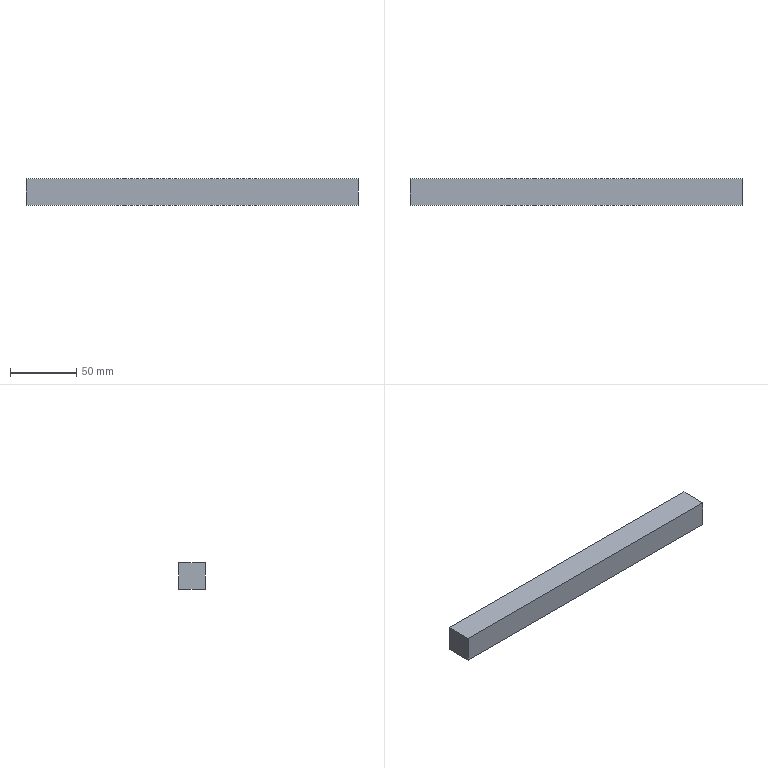Part | STEP file | 122_id1162_x_t | 1 solid | 6 faces | box 250 x 20 x 20 mm | volume 100000 mm3 | plane 6
STEP:
#1=CARTESIAN_POINT('',(0.,0.,0.));
#2=DIRECTION('',(0.,0.,1.));
#3=DIRECTION('',(1.,0.,0.));
#4=AXIS2_PLACEMENT_3D('',#1,#2,#3);
#5=CARTESIAN_POINT('',(94.,701.,120.));
#6=VERTEX_POINT('',#5);
#7=CARTESIAN_POINT('',(-156.,701.,120.));
#8=VERTEX_POINT('',#7);
#9=CARTESIAN_POINT('',(-31.,701.,120.));
#10=DIRECTION('',(-1.,0.,0.));
#11=VECTOR('',#10,1.);
#12=LINE('',#9,#11);
#13=CARTESIAN_POINT('',(-31.,711.,120.));
#14=DIRECTION('',(0.,0.,1.));
#15=DIRECTION('',(1.,0.,0.));
#16=AXIS2_PLACEMENT_3D('',#13,#14,#15);
#17=PLANE('',#16);
#18=CARTESIAN_POINT('',(0.,-10.));
#19=DIRECTION('',(-1.,0.));
#20=VECTOR('',#19,1.);
#21=LINE('',#18,#20);
#22=(GEOMETRIC_REPRESENTATION_CONTEXT(2)PARAMETRIC_REPRESENTATION_CONTEXT()REPRESENTATION_CONTEXT('',''));
#23=DEFINITIONAL_REPRESENTATION('',(#21),#22);
#24=PCURVE('',#17,#23);
#25=CARTESIAN_POINT('',(-31.,701.,100.));
#26=DIRECTION('',(0.,-1.,0.));
#27=DIRECTION('',(0.,0.,-1.));
#28=AXIS2_PLACEMENT_3D('',#25,#26,#27);
#29=PLANE('',#28);
#30=CARTESIAN_POINT('',(-20.,0.));
#31=DIRECTION('',(0.,-1.));
#32=VECTOR('',#31,1.);
#33=LINE('',#30,#32);
#34=(GEOMETRIC_REPRESENTATION_CONTEXT(2)PARAMETRIC_REPRESENTATION_CONTEXT()REPRESENTATION_CONTEXT('',''));
#35=DEFINITIONAL_REPRESENTATION('',(#33),#34);
#36=PCURVE('',#29,#35);
#37=SURFACE_CURVE('',#12,(#24,#36),.PCURVE_S1.);
#38=EDGE_CURVE('',#6,#8,#37,.T.);
#39=ORIENTED_EDGE('',*,*,#38,.F.);
#40=CARTESIAN_POINT('',(94.,721.,120.));
#41=VERTEX_POINT('',#40);
#42=CARTESIAN_POINT('',(94.,711.,120.));
#43=DIRECTION('',(0.,-1.,0.));
#44=VECTOR('',#43,1.);
#45=LINE('',#42,#44);
#46=CARTESIAN_POINT('',(125.,0.));
#47=DIRECTION('',(0.,-1.));
#48=VECTOR('',#47,1.);
#49=LINE('',#46,#48);
#50=(GEOMETRIC_REPRESENTATION_CONTEXT(2)PARAMETRIC_REPRESENTATION_CONTEXT()REPRESENTATION_CONTEXT('',''));
#51=DEFINITIONAL_REPRESENTATION('',(#49),#50);
#52=PCURVE('',#17,#51);
#53=CARTESIAN_POINT('',(94.,711.,100.));
#54=DIRECTION('',(1.,0.,0.));
#55=DIRECTION('',(0.,0.,-1.));
#56=AXIS2_PLACEMENT_3D('',#53,#54,#55);
#57=PLANE('',#56);
#58=CARTESIAN_POINT('',(-20.,0.));
#59=DIRECTION('',(0.,-1.));
#60=VECTOR('',#59,1.);
#61=LINE('',#58,#60);
#62=(GEOMETRIC_REPRESENTATION_CONTEXT(2)PARAMETRIC_REPRESENTATION_CONTEXT()REPRESENTATION_CONTEXT('',''));
#63=DEFINITIONAL_REPRESENTATION('',(#61),#62);
#64=PCURVE('',#57,#63);
#65=SURFACE_CURVE('',#45,(#52,#64),.PCURVE_S1.);
#66=EDGE_CURVE('',#41,#6,#65,.T.);
#67=ORIENTED_EDGE('',*,*,#66,.F.);
#68=CARTESIAN_POINT('',(-156.,721.,120.));
#69=VERTEX_POINT('',#68);
#70=CARTESIAN_POINT('',(-31.,721.,120.));
#71=DIRECTION('',(1.,0.,0.));
#72=VECTOR('',#71,1.);
#73=LINE('',#70,#72);
#74=CARTESIAN_POINT('',(0.,10.));
#75=DIRECTION('',(1.,0.));
#76=VECTOR('',#75,1.);
#77=LINE('',#74,#76);
#78=(GEOMETRIC_REPRESENTATION_CONTEXT(2)PARAMETRIC_REPRESENTATION_CONTEXT()REPRESENTATION_CONTEXT('',''));
#79=DEFINITIONAL_REPRESENTATION('',(#77),#78);
#80=PCURVE('',#17,#79);
#81=CARTESIAN_POINT('',(-31.,721.,100.));
#82=DIRECTION('',(0.,1.,0.));
#83=DIRECTION('',(0.,0.,1.));
#84=AXIS2_PLACEMENT_3D('',#81,#82,#83);
#85=PLANE('',#84);
#86=CARTESIAN_POINT('',(20.,0.));
#87=DIRECTION('',(0.,1.));
#88=VECTOR('',#87,1.);
#89=LINE('',#86,#88);
#90=(GEOMETRIC_REPRESENTATION_CONTEXT(2)PARAMETRIC_REPRESENTATION_CONTEXT()REPRESENTATION_CONTEXT('',''));
#91=DEFINITIONAL_REPRESENTATION('',(#89),#90);
#92=PCURVE('',#85,#91);
#93=SURFACE_CURVE('',#73,(#80,#92),.PCURVE_S1.);
#94=EDGE_CURVE('',#69,#41,#93,.T.);
#95=ORIENTED_EDGE('',*,*,#94,.F.);
#96=CARTESIAN_POINT('',(-156.,711.,120.));
#97=DIRECTION('',(0.,1.,0.));
#98=VECTOR('',#97,1.);
#99=LINE('',#96,#98);
#100=CARTESIAN_POINT('',(-125.,0.));
#101=DIRECTION('',(0.,1.));
#102=VECTOR('',#101,1.);
#103=LINE('',#100,#102);
#104=(GEOMETRIC_REPRESENTATION_CONTEXT(2)PARAMETRIC_REPRESENTATION_CONTEXT()REPRESENTATION_CONTEXT('',''));
#105=DEFINITIONAL_REPRESENTATION('',(#103),#104);
#106=PCURVE('',#17,#105);
#107=CARTESIAN_POINT('',(-156.,711.,100.));
#108=DIRECTION('',(-1.,0.,0.));
#109=DIRECTION('',(0.,0.,1.));
#110=AXIS2_PLACEMENT_3D('',#107,#108,#109);
#111=PLANE('',#110);
#112=CARTESIAN_POINT('',(20.,0.));
#113=DIRECTION('',(0.,1.));
#114=VECTOR('',#113,1.);
#115=LINE('',#112,#114);
#116=(GEOMETRIC_REPRESENTATION_CONTEXT(2)PARAMETRIC_REPRESENTATION_CONTEXT()REPRESENTATION_CONTEXT('',''));
#117=DEFINITIONAL_REPRESENTATION('',(#115),#116);
#118=PCURVE('',#111,#117);
#119=SURFACE_CURVE('',#99,(#106,#118),.PCURVE_S1.);
#120=EDGE_CURVE('',#8,#69,#119,.T.);
#121=ORIENTED_EDGE('',*,*,#120,.F.);
#122=EDGE_LOOP('',(#39,#67,#95,#121));
#123=FACE_BOUND('',#122,.T.);
#124=ADVANCED_FACE('',(#123),#17,.T.);
#125=CARTESIAN_POINT('',(94.,701.,100.));
#126=VERTEX_POINT('',#125);
#127=CARTESIAN_POINT('',(94.,701.,100.));
#128=DIRECTION('',(0.,0.,1.));
#129=VECTOR('',#128,1.);
#130=LINE('',#127,#129);
#131=CARTESIAN_POINT('',(0.,125.));
#132=DIRECTION('',(-1.,0.));
#133=VECTOR('',#132,1.);
#134=LINE('',#131,#133);
#135=(GEOMETRIC_REPRESENTATION_CONTEXT(2)PARAMETRIC_REPRESENTATION_CONTEXT()REPRESENTATION_CONTEXT('',''));
#136=DEFINITIONAL_REPRESENTATION('',(#134),#135);
#137=PCURVE('',#29,#136);
#138=CARTESIAN_POINT('',(0.,-10.));
#139=DIRECTION('',(-1.,0.));
#140=VECTOR('',#139,1.);
#141=LINE('',#138,#140);
#142=(GEOMETRIC_REPRESENTATION_CONTEXT(2)PARAMETRIC_REPRESENTATION_CONTEXT()REPRESENTATION_CONTEXT('',''));
#143=DEFINITIONAL_REPRESENTATION('',(#141),#142);
#144=PCURVE('',#57,#143);
#145=SURFACE_CURVE('',#130,(#137,#144),.PCURVE_S1.);
#146=EDGE_CURVE('',#126,#6,#145,.T.);
#147=ORIENTED_EDGE('',*,*,#146,.T.);
#148=ORIENTED_EDGE('',*,*,#38,.T.);
#149=CARTESIAN_POINT('',(-156.,701.,100.));
#150=VERTEX_POINT('',#149);
#151=CARTESIAN_POINT('',(-156.,701.,100.));
#152=DIRECTION('',(0.,0.,1.));
#153=VECTOR('',#152,1.);
#154=LINE('',#151,#153);
#155=CARTESIAN_POINT('',(0.,-125.));
#156=DIRECTION('',(-1.,0.));
#157=VECTOR('',#156,1.);
#158=LINE('',#155,#157);
#159=(GEOMETRIC_REPRESENTATION_CONTEXT(2)PARAMETRIC_REPRESENTATION_CONTEXT()REPRESENTATION_CONTEXT('',''));
#160=DEFINITIONAL_REPRESENTATION('',(#158),#159);
#161=PCURVE('',#29,#160);
#162=CARTESIAN_POINT('',(0.,-10.));
#163=DIRECTION('',(1.,0.));
#164=VECTOR('',#163,1.);
#165=LINE('',#162,#164);
#166=(GEOMETRIC_REPRESENTATION_CONTEXT(2)PARAMETRIC_REPRESENTATION_CONTEXT()REPRESENTATION_CONTEXT('',''));
#167=DEFINITIONAL_REPRESENTATION('',(#165),#166);
#168=PCURVE('',#111,#167);
#169=SURFACE_CURVE('',#154,(#161,#168),.PCURVE_S1.);
#170=EDGE_CURVE('',#150,#8,#169,.T.);
#171=ORIENTED_EDGE('',*,*,#170,.F.);
#172=CARTESIAN_POINT('',(-31.,701.,100.));
#173=DIRECTION('',(1.,0.,0.));
#174=VECTOR('',#173,1.);
#175=LINE('',#172,#174);
#176=CARTESIAN_POINT('',(0.,0.));
#177=DIRECTION('',(0.,1.));
#178=VECTOR('',#177,1.);
#179=LINE('',#176,#178);
#180=(GEOMETRIC_REPRESENTATION_CONTEXT(2)PARAMETRIC_REPRESENTATION_CONTEXT()REPRESENTATION_CONTEXT('',''));
#181=DEFINITIONAL_REPRESENTATION('',(#179),#180);
#182=PCURVE('',#29,#181);
#183=CARTESIAN_POINT('',(-31.,711.,100.));
#184=DIRECTION('',(0.,0.,-1.));
#185=DIRECTION('',(-1.,0.,0.));
#186=AXIS2_PLACEMENT_3D('',#183,#184,#185);
#187=PLANE('',#186);
#188=CARTESIAN_POINT('',(0.,-10.));
#189=DIRECTION('',(-1.,0.));
#190=VECTOR('',#189,1.);
#191=LINE('',#188,#190);
#192=(GEOMETRIC_REPRESENTATION_CONTEXT(2)PARAMETRIC_REPRESENTATION_CONTEXT()REPRESENTATION_CONTEXT('',''));
#193=DEFINITIONAL_REPRESENTATION('',(#191),#192);
#194=PCURVE('',#187,#193);
#195=SURFACE_CURVE('',#175,(#182,#194),.PCURVE_S1.);
#196=EDGE_CURVE('',#150,#126,#195,.T.);
#197=ORIENTED_EDGE('',*,*,#196,.T.);
#198=EDGE_LOOP('',(#147,#148,#171,#197));
#199=FACE_BOUND('',#198,.T.);
#200=ADVANCED_FACE('',(#199),#29,.T.);
#201=ORIENTED_EDGE('',*,*,#170,.T.);
#202=ORIENTED_EDGE('',*,*,#120,.T.);
#203=CARTESIAN_POINT('',(-156.,721.,100.));
#204=VERTEX_POINT('',#203);
#205=CARTESIAN_POINT('',(-156.,721.,100.));
#206=DIRECTION('',(0.,0.,1.));
#207=VECTOR('',#206,1.);
#208=LINE('',#205,#207);
#209=CARTESIAN_POINT('',(0.,10.));
#210=DIRECTION('',(1.,0.));
#211=VECTOR('',#210,1.);
#212=LINE('',#209,#211);
#213=(GEOMETRIC_REPRESENTATION_CONTEXT(2)PARAMETRIC_REPRESENTATION_CONTEXT()REPRESENTATION_CONTEXT('',''));
#214=DEFINITIONAL_REPRESENTATION('',(#212),#213);
#215=PCURVE('',#111,#214);
#216=CARTESIAN_POINT('',(0.,-125.));
#217=DIRECTION('',(1.,0.));
#218=VECTOR('',#217,1.);
#219=LINE('',#216,#218);
#220=(GEOMETRIC_REPRESENTATION_CONTEXT(2)PARAMETRIC_REPRESENTATION_CONTEXT()REPRESENTATION_CONTEXT('',''));
#221=DEFINITIONAL_REPRESENTATION('',(#219),#220);
#222=PCURVE('',#85,#221);
#223=SURFACE_CURVE('',#208,(#215,#222),.PCURVE_S1.);
#224=EDGE_CURVE('',#204,#69,#223,.T.);
#225=ORIENTED_EDGE('',*,*,#224,.F.);
#226=CARTESIAN_POINT('',(-156.,711.,100.));
#227=DIRECTION('',(0.,-1.,0.));
#228=VECTOR('',#227,1.);
#229=LINE('',#226,#228);
#230=CARTESIAN_POINT('',(0.,0.));
#231=DIRECTION('',(0.,-1.));
#232=VECTOR('',#231,1.);
#233=LINE('',#230,#232);
#234=(GEOMETRIC_REPRESENTATION_CONTEXT(2)PARAMETRIC_REPRESENTATION_CONTEXT()REPRESENTATION_CONTEXT('',''));
#235=DEFINITIONAL_REPRESENTATION('',(#233),#234);
#236=PCURVE('',#111,#235);
#237=CARTESIAN_POINT('',(125.,0.));
#238=DIRECTION('',(0.,-1.));
#239=VECTOR('',#238,1.);
#240=LINE('',#237,#239);
#241=(GEOMETRIC_REPRESENTATION_CONTEXT(2)PARAMETRIC_REPRESENTATION_CONTEXT()REPRESENTATION_CONTEXT('',''));
#242=DEFINITIONAL_REPRESENTATION('',(#240),#241);
#243=PCURVE('',#187,#242);
#244=SURFACE_CURVE('',#229,(#236,#243),.PCURVE_S1.);
#245=EDGE_CURVE('',#204,#150,#244,.T.);
#246=ORIENTED_EDGE('',*,*,#245,.T.);
#247=EDGE_LOOP('',(#201,#202,#225,#246));
#248=FACE_BOUND('',#247,.T.);
#249=ADVANCED_FACE('',(#248),#111,.T.);
#250=ORIENTED_EDGE('',*,*,#224,.T.);
#251=ORIENTED_EDGE('',*,*,#94,.T.);
#252=CARTESIAN_POINT('',(94.,721.,100.));
#253=VERTEX_POINT('',#252);
#254=CARTESIAN_POINT('',(94.,721.,100.));
#255=DIRECTION('',(0.,0.,1.));
#256=VECTOR('',#255,1.);
#257=LINE('',#254,#256);
#258=CARTESIAN_POINT('',(0.,125.));
#259=DIRECTION('',(1.,0.));
#260=VECTOR('',#259,1.);
#261=LINE('',#258,#260);
#262=(GEOMETRIC_REPRESENTATION_CONTEXT(2)PARAMETRIC_REPRESENTATION_CONTEXT()REPRESENTATION_CONTEXT('',''));
#263=DEFINITIONAL_REPRESENTATION('',(#261),#262);
#264=PCURVE('',#85,#263);
#265=CARTESIAN_POINT('',(0.,10.));
#266=DIRECTION('',(-1.,0.));
#267=VECTOR('',#266,1.);
#268=LINE('',#265,#267);
#269=(GEOMETRIC_REPRESENTATION_CONTEXT(2)PARAMETRIC_REPRESENTATION_CONTEXT()REPRESENTATION_CONTEXT('',''));
#270=DEFINITIONAL_REPRESENTATION('',(#268),#269);
#271=PCURVE('',#57,#270);
#272=SURFACE_CURVE('',#257,(#264,#271),.PCURVE_S1.);
#273=EDGE_CURVE('',#253,#41,#272,.T.);
#274=ORIENTED_EDGE('',*,*,#273,.F.);
#275=CARTESIAN_POINT('',(-31.,721.,100.));
#276=DIRECTION('',(-1.,0.,0.));
#277=VECTOR('',#276,1.);
#278=LINE('',#275,#277);
#279=CARTESIAN_POINT('',(0.,0.));
#280=DIRECTION('',(0.,-1.));
#281=VECTOR('',#280,1.);
#282=LINE('',#279,#281);
#283=(GEOMETRIC_REPRESENTATION_CONTEXT(2)PARAMETRIC_REPRESENTATION_CONTEXT()REPRESENTATION_CONTEXT('',''));
#284=DEFINITIONAL_REPRESENTATION('',(#282),#283);
#285=PCURVE('',#85,#284);
#286=CARTESIAN_POINT('',(0.,10.));
#287=DIRECTION('',(1.,0.));
#288=VECTOR('',#287,1.);
#289=LINE('',#286,#288);
#290=(GEOMETRIC_REPRESENTATION_CONTEXT(2)PARAMETRIC_REPRESENTATION_CONTEXT()REPRESENTATION_CONTEXT('',''));
#291=DEFINITIONAL_REPRESENTATION('',(#289),#290);
#292=PCURVE('',#187,#291);
#293=SURFACE_CURVE('',#278,(#285,#292),.PCURVE_S1.);
#294=EDGE_CURVE('',#253,#204,#293,.T.);
#295=ORIENTED_EDGE('',*,*,#294,.T.);
#296=EDGE_LOOP('',(#250,#251,#274,#295));
#297=FACE_BOUND('',#296,.T.);
#298=ADVANCED_FACE('',(#297),#85,.T.);
#299=CARTESIAN_POINT('',(94.,711.,100.));
#300=DIRECTION('',(0.,1.,0.));
#301=VECTOR('',#300,1.);
#302=LINE('',#299,#301);
#303=CARTESIAN_POINT('',(-125.,0.));
#304=DIRECTION('',(0.,1.));
#305=VECTOR('',#304,1.);
#306=LINE('',#303,#305);
#307=(GEOMETRIC_REPRESENTATION_CONTEXT(2)PARAMETRIC_REPRESENTATION_CONTEXT()REPRESENTATION_CONTEXT('',''));
#308=DEFINITIONAL_REPRESENTATION('',(#306),#307);
#309=PCURVE('',#187,#308);
#310=CARTESIAN_POINT('',(0.,0.));
#311=DIRECTION('',(0.,1.));
#312=VECTOR('',#311,1.);
#313=LINE('',#310,#312);
#314=(GEOMETRIC_REPRESENTATION_CONTEXT(2)PARAMETRIC_REPRESENTATION_CONTEXT()REPRESENTATION_CONTEXT('',''));
#315=DEFINITIONAL_REPRESENTATION('',(#313),#314);
#316=PCURVE('',#57,#315);
#317=SURFACE_CURVE('',#302,(#309,#316),.PCURVE_S1.);
#318=EDGE_CURVE('',#126,#253,#317,.T.);
#319=ORIENTED_EDGE('',*,*,#318,.F.);
#320=ORIENTED_EDGE('',*,*,#196,.F.);
#321=ORIENTED_EDGE('',*,*,#245,.F.);
#322=ORIENTED_EDGE('',*,*,#294,.F.);
#323=EDGE_LOOP('',(#319,#320,#321,#322));
#324=FACE_BOUND('',#323,.T.);
#325=ADVANCED_FACE('',(#324),#187,.T.);
#326=ORIENTED_EDGE('',*,*,#318,.T.);
#327=ORIENTED_EDGE('',*,*,#273,.T.);
#328=ORIENTED_EDGE('',*,*,#66,.T.);
#329=ORIENTED_EDGE('',*,*,#146,.F.);
#330=EDGE_LOOP('',(#326,#327,#328,#329));
#331=FACE_BOUND('',#330,.T.);
#332=ADVANCED_FACE('',(#331),#57,.T.);
#333=CLOSED_SHELL('',(#124,#200,#249,#298,#325,#332));
#334=MANIFOLD_SOLID_BREP('',#333);
#335=(LENGTH_UNIT()NAMED_UNIT(*)SI_UNIT(.MILLI.,.METRE.));
#336=UNCERTAINTY_MEASURE_WITH_UNIT(LENGTH_MEASURE(0.0000001),#335,'','');
#337=(NAMED_UNIT(*)PLANE_ANGLE_UNIT()SI_UNIT($,.RADIAN.));
#338=(NAMED_UNIT(*)SI_UNIT($,.STERADIAN.)SOLID_ANGLE_UNIT());
#339=(GEOMETRIC_REPRESENTATION_CONTEXT(3)GLOBAL_UNCERTAINTY_ASSIGNED_CONTEXT((#336))GLOBAL_UNIT_ASSIGNED_CONTEXT((#335,#337,#338))REPRESENTATION_CONTEXT('',''));
#340=ADVANCED_BREP_SHAPE_REPRESENTATION('',(#4,#334),#339);